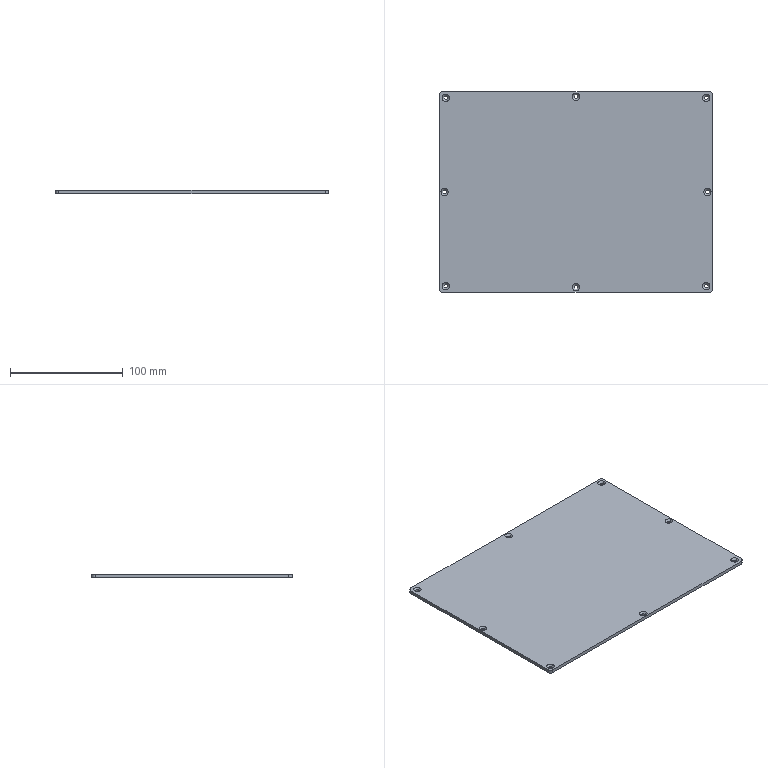Part | SolidWorks | features Extrusion 1, Fillet 1, HoleWzd 1 | 1 solid | 42 faces | box 242 x 178 x 3 mm | volume 128843 mm3 | cylinder 20 | cone 16 | plane 6 | commonest cylinder face diameters 3.4 x16 6 x4
STEP:
#1=CARTESIAN_POINT('',(-1.7,84.5,1.4));
#2=VERTEX_POINT('',#1);
#3=CARTESIAN_POINT('',(1.7,84.5,1.4));
#4=VERTEX_POINT('',#3);
#5=CARTESIAN_POINT('',(0.,84.5,1.4));
#6=DIRECTION('',(0.,0.,1.));
#7=DIRECTION('',(1.,0.,0.));
#8=AXIS2_PLACEMENT_3D('',#5,#6,#7);
#9=CIRCLE('',#8,1.7);
#10=EDGE_CURVE('',#2,#4,#9,.T.);
#11=ORIENTED_EDGE('',*,*,#10,.F.);
#12=CARTESIAN_POINT('',(-3.3,84.5,3.));
#13=VERTEX_POINT('',#12);
#14=CARTESIAN_POINT('',(-3.3,84.5,3.));
#15=DIRECTION('',(-0.7071,0.,0.7071));
#16=VECTOR('',#15,1000.);
#17=LINE('',#14,#16);
#18=EDGE_CURVE('',#2,#13,#17,.T.);
#19=ORIENTED_EDGE('',*,*,#18,.T.);
#20=CARTESIAN_POINT('',(3.3,84.5,3.));
#21=VERTEX_POINT('',#20);
#22=CARTESIAN_POINT('',(0.,84.5,3.));
#23=DIRECTION('',(0.,0.,1.));
#24=DIRECTION('',(1.,0.,0.));
#25=AXIS2_PLACEMENT_3D('',#22,#23,#24);
#26=CIRCLE('',#25,3.3);
#27=EDGE_CURVE('',#13,#21,#26,.T.);
#28=ORIENTED_EDGE('',*,*,#27,.T.);
#29=CARTESIAN_POINT('',(3.3,84.5,3.));
#30=DIRECTION('',(0.7071,0.,0.7071));
#31=VECTOR('',#30,1000.);
#32=LINE('',#29,#31);
#33=EDGE_CURVE('',#4,#21,#32,.T.);
#34=ORIENTED_EDGE('',*,*,#33,.F.);
#35=EDGE_LOOP('',(#11,#19,#28,#34));
#36=FACE_OUTER_BOUND('',#35,.T.);
#37=CARTESIAN_POINT('',(0.,84.5,3.));
#38=DIRECTION('',(0.,0.,1.));
#39=DIRECTION('',(1.,0.,0.));
#40=AXIS2_PLACEMENT_3D('',#37,#38,#39);
#41=CONICAL_SURFACE('',#40,3.3,0.7854);
#42=ADVANCED_FACE('',(#36),#41,.F.);
#43=CARTESIAN_POINT('',(-1.7,84.5,0.));
#44=VERTEX_POINT('',#43);
#45=CARTESIAN_POINT('',(1.7,84.5,0.));
#46=VERTEX_POINT('',#45);
#47=CARTESIAN_POINT('',(0.,84.5,0.));
#48=DIRECTION('',(0.,0.,1.));
#49=DIRECTION('',(1.,0.,0.));
#50=AXIS2_PLACEMENT_3D('',#47,#48,#49);
#51=CIRCLE('',#50,1.7);
#52=EDGE_CURVE('',#44,#46,#51,.T.);
#53=ORIENTED_EDGE('',*,*,#52,.F.);
#54=CARTESIAN_POINT('',(-1.7,84.5,3.));
#55=DIRECTION('',(0.,0.,1.));
#56=VECTOR('',#55,1000.);
#57=LINE('',#54,#56);
#58=EDGE_CURVE('',#44,#2,#57,.T.);
#59=ORIENTED_EDGE('',*,*,#58,.T.);
#60=ORIENTED_EDGE('',*,*,#10,.T.);
#61=CARTESIAN_POINT('',(1.7,84.5,3.));
#62=DIRECTION('',(0.,0.,1.));
#63=VECTOR('',#62,1000.);
#64=LINE('',#61,#63);
#65=EDGE_CURVE('',#46,#4,#64,.T.);
#66=ORIENTED_EDGE('',*,*,#65,.F.);
#67=EDGE_LOOP('',(#53,#59,#60,#66));
#68=FACE_OUTER_BOUND('',#67,.T.);
#69=CARTESIAN_POINT('',(0.,84.5,3.));
#70=DIRECTION('',(0.,0.,1.));
#71=DIRECTION('',(1.,0.,0.));
#72=AXIS2_PLACEMENT_3D('',#69,#70,#71);
#73=CYLINDRICAL_SURFACE('',#72,1.7);
#74=ADVANCED_FACE('',(#68),#73,.F.);
#75=CARTESIAN_POINT('',(-118.2,0.,1.4));
#76=VERTEX_POINT('',#75);
#77=CARTESIAN_POINT('',(-114.8,0.,1.4));
#78=VERTEX_POINT('',#77);
#79=CARTESIAN_POINT('',(-116.5,0.,1.4));
#80=DIRECTION('',(0.,0.,1.));
#81=DIRECTION('',(1.,0.,0.));
#82=AXIS2_PLACEMENT_3D('',#79,#80,#81);
#83=CIRCLE('',#82,1.7);
#84=EDGE_CURVE('',#76,#78,#83,.T.);
#85=ORIENTED_EDGE('',*,*,#84,.F.);
#86=CARTESIAN_POINT('',(-119.8,0.,3.));
#87=VERTEX_POINT('',#86);
#88=CARTESIAN_POINT('',(-119.8,0.,3.));
#89=DIRECTION('',(-0.7071,0.,0.7071));
#90=VECTOR('',#89,1000.);
#91=LINE('',#88,#90);
#92=EDGE_CURVE('',#76,#87,#91,.T.);
#93=ORIENTED_EDGE('',*,*,#92,.T.);
#94=CARTESIAN_POINT('',(-113.2,0.,3.));
#95=VERTEX_POINT('',#94);
#96=CARTESIAN_POINT('',(-116.5,0.,3.));
#97=DIRECTION('',(0.,0.,1.));
#98=DIRECTION('',(1.,0.,0.));
#99=AXIS2_PLACEMENT_3D('',#96,#97,#98);
#100=CIRCLE('',#99,3.3);
#101=EDGE_CURVE('',#87,#95,#100,.T.);
#102=ORIENTED_EDGE('',*,*,#101,.T.);
#103=CARTESIAN_POINT('',(-113.2,0.,3.));
#104=DIRECTION('',(0.7071,0.,0.7071));
#105=VECTOR('',#104,1000.);
#106=LINE('',#103,#105);
#107=EDGE_CURVE('',#78,#95,#106,.T.);
#108=ORIENTED_EDGE('',*,*,#107,.F.);
#109=EDGE_LOOP('',(#85,#93,#102,#108));
#110=FACE_OUTER_BOUND('',#109,.T.);
#111=CARTESIAN_POINT('',(-116.5,0.,3.));
#112=DIRECTION('',(0.,0.,1.));
#113=DIRECTION('',(1.,0.,0.));
#114=AXIS2_PLACEMENT_3D('',#111,#112,#113);
#115=CONICAL_SURFACE('',#114,3.3,0.7854);
#116=ADVANCED_FACE('',(#110),#115,.F.);
#117=CARTESIAN_POINT('',(-118.2,0.,0.));
#118=VERTEX_POINT('',#117);
#119=CARTESIAN_POINT('',(-114.8,0.,0.));
#120=VERTEX_POINT('',#119);
#121=CARTESIAN_POINT('',(-116.5,0.,0.));
#122=DIRECTION('',(0.,0.,1.));
#123=DIRECTION('',(1.,0.,0.));
#124=AXIS2_PLACEMENT_3D('',#121,#122,#123);
#125=CIRCLE('',#124,1.7);
#126=EDGE_CURVE('',#118,#120,#125,.T.);
#127=ORIENTED_EDGE('',*,*,#126,.F.);
#128=CARTESIAN_POINT('',(-118.2,0.,3.));
#129=DIRECTION('',(0.,0.,1.));
#130=VECTOR('',#129,1000.);
#131=LINE('',#128,#130);
#132=EDGE_CURVE('',#118,#76,#131,.T.);
#133=ORIENTED_EDGE('',*,*,#132,.T.);
#134=ORIENTED_EDGE('',*,*,#84,.T.);
#135=CARTESIAN_POINT('',(-114.8,0.,3.));
#136=DIRECTION('',(0.,0.,1.));
#137=VECTOR('',#136,1000.);
#138=LINE('',#135,#137);
#139=EDGE_CURVE('',#120,#78,#138,.T.);
#140=ORIENTED_EDGE('',*,*,#139,.F.);
#141=EDGE_LOOP('',(#127,#133,#134,#140));
#142=FACE_OUTER_BOUND('',#141,.T.);
#143=CARTESIAN_POINT('',(-116.5,0.,3.));
#144=DIRECTION('',(0.,0.,1.));
#145=DIRECTION('',(1.,0.,0.));
#146=AXIS2_PLACEMENT_3D('',#143,#144,#145);
#147=CYLINDRICAL_SURFACE('',#146,1.7);
#148=ADVANCED_FACE('',(#142),#147,.F.);
#149=CARTESIAN_POINT('',(-1.7,-84.5,1.4));
#150=VERTEX_POINT('',#149);
#151=CARTESIAN_POINT('',(1.7,-84.5,1.4));
#152=VERTEX_POINT('',#151);
#153=CARTESIAN_POINT('',(0.,-84.5,1.4));
#154=DIRECTION('',(0.,0.,1.));
#155=DIRECTION('',(1.,0.,0.));
#156=AXIS2_PLACEMENT_3D('',#153,#154,#155);
#157=CIRCLE('',#156,1.7);
#158=EDGE_CURVE('',#150,#152,#157,.T.);
#159=ORIENTED_EDGE('',*,*,#158,.F.);
#160=CARTESIAN_POINT('',(-3.3,-84.5,3.));
#161=VERTEX_POINT('',#160);
#162=CARTESIAN_POINT('',(-3.3,-84.5,3.));
#163=DIRECTION('',(-0.7071,0.,0.7071));
#164=VECTOR('',#163,1000.);
#165=LINE('',#162,#164);
#166=EDGE_CURVE('',#150,#161,#165,.T.);
#167=ORIENTED_EDGE('',*,*,#166,.T.);
#168=CARTESIAN_POINT('',(3.3,-84.5,3.));
#169=VERTEX_POINT('',#168);
#170=CARTESIAN_POINT('',(0.,-84.5,3.));
#171=DIRECTION('',(0.,0.,1.));
#172=DIRECTION('',(1.,0.,0.));
#173=AXIS2_PLACEMENT_3D('',#170,#171,#172);
#174=CIRCLE('',#173,3.3);
#175=EDGE_CURVE('',#161,#169,#174,.T.);
#176=ORIENTED_EDGE('',*,*,#175,.T.);
#177=CARTESIAN_POINT('',(3.3,-84.5,3.));
#178=DIRECTION('',(0.7071,0.,0.7071));
#179=VECTOR('',#178,1000.);
#180=LINE('',#177,#179);
#181=EDGE_CURVE('',#152,#169,#180,.T.);
#182=ORIENTED_EDGE('',*,*,#181,.F.);
#183=EDGE_LOOP('',(#159,#167,#176,#182));
#184=FACE_OUTER_BOUND('',#183,.T.);
#185=CARTESIAN_POINT('',(0.,-84.5,3.));
#186=DIRECTION('',(0.,0.,1.));
#187=DIRECTION('',(1.,0.,0.));
#188=AXIS2_PLACEMENT_3D('',#185,#186,#187);
#189=CONICAL_SURFACE('',#188,3.3,0.7854);
#190=ADVANCED_FACE('',(#184),#189,.F.);
#191=CARTESIAN_POINT('',(-1.7,-84.5,0.));
#192=VERTEX_POINT('',#191);
#193=CARTESIAN_POINT('',(1.7,-84.5,0.));
#194=VERTEX_POINT('',#193);
#195=CARTESIAN_POINT('',(0.,-84.5,0.));
#196=DIRECTION('',(0.,0.,1.));
#197=DIRECTION('',(1.,0.,0.));
#198=AXIS2_PLACEMENT_3D('',#195,#196,#197);
#199=CIRCLE('',#198,1.7);
#200=EDGE_CURVE('',#192,#194,#199,.T.);
#201=ORIENTED_EDGE('',*,*,#200,.F.);
#202=CARTESIAN_POINT('',(-1.7,-84.5,3.));
#203=DIRECTION('',(0.,0.,1.));
#204=VECTOR('',#203,1000.);
#205=LINE('',#202,#204);
#206=EDGE_CURVE('',#192,#150,#205,.T.);
#207=ORIENTED_EDGE('',*,*,#206,.T.);
#208=ORIENTED_EDGE('',*,*,#158,.T.);
#209=CARTESIAN_POINT('',(1.7,-84.5,3.));
#210=DIRECTION('',(0.,0.,1.));
#211=VECTOR('',#210,1000.);
#212=LINE('',#209,#211);
#213=EDGE_CURVE('',#194,#152,#212,.T.);
#214=ORIENTED_EDGE('',*,*,#213,.F.);
#215=EDGE_LOOP('',(#201,#207,#208,#214));
#216=FACE_OUTER_BOUND('',#215,.T.);
#217=CARTESIAN_POINT('',(0.,-84.5,3.));
#218=DIRECTION('',(0.,0.,1.));
#219=DIRECTION('',(1.,0.,0.));
#220=AXIS2_PLACEMENT_3D('',#217,#218,#219);
#221=CYLINDRICAL_SURFACE('',#220,1.7);
#222=ADVANCED_FACE('',(#216),#221,.F.);
#223=CARTESIAN_POINT('',(114.8,0.,1.4));
#224=VERTEX_POINT('',#223);
#225=CARTESIAN_POINT('',(118.2,0.,1.4));
#226=VERTEX_POINT('',#225);
#227=CARTESIAN_POINT('',(116.5,0.,1.4));
#228=DIRECTION('',(0.,0.,1.));
#229=DIRECTION('',(1.,0.,0.));
#230=AXIS2_PLACEMENT_3D('',#227,#228,#229);
#231=CIRCLE('',#230,1.7);
#232=EDGE_CURVE('',#224,#226,#231,.T.);
#233=ORIENTED_EDGE('',*,*,#232,.F.);
#234=CARTESIAN_POINT('',(113.2,0.,3.));
#235=VERTEX_POINT('',#234);
#236=CARTESIAN_POINT('',(113.2,0.,3.));
#237=DIRECTION('',(-0.7071,0.,0.7071));
#238=VECTOR('',#237,1000.);
#239=LINE('',#236,#238);
#240=EDGE_CURVE('',#224,#235,#239,.T.);
#241=ORIENTED_EDGE('',*,*,#240,.T.);
#242=CARTESIAN_POINT('',(119.8,0.,3.));
#243=VERTEX_POINT('',#242);
#244=CARTESIAN_POINT('',(116.5,0.,3.));
#245=DIRECTION('',(0.,0.,1.));
#246=DIRECTION('',(1.,0.,0.));
#247=AXIS2_PLACEMENT_3D('',#244,#245,#246);
#248=CIRCLE('',#247,3.3);
#249=EDGE_CURVE('',#235,#243,#248,.T.);
#250=ORIENTED_EDGE('',*,*,#249,.T.);
#251=CARTESIAN_POINT('',(119.8,0.,3.));
#252=DIRECTION('',(0.7071,0.,0.7071));
#253=VECTOR('',#252,1000.);
#254=LINE('',#251,#253);
#255=EDGE_CURVE('',#226,#243,#254,.T.);
#256=ORIENTED_EDGE('',*,*,#255,.F.);
#257=EDGE_LOOP('',(#233,#241,#250,#256));
#258=FACE_OUTER_BOUND('',#257,.T.);
#259=CARTESIAN_POINT('',(116.5,0.,3.));
#260=DIRECTION('',(0.,0.,1.));
#261=DIRECTION('',(1.,0.,0.));
#262=AXIS2_PLACEMENT_3D('',#259,#260,#261);
#263=CONICAL_SURFACE('',#262,3.3,0.7854);
#264=ADVANCED_FACE('',(#258),#263,.F.);
#265=CARTESIAN_POINT('',(114.8,0.,0.));
#266=VERTEX_POINT('',#265);
#267=CARTESIAN_POINT('',(118.2,0.,0.));
#268=VERTEX_POINT('',#267);
#269=CARTESIAN_POINT('',(116.5,0.,0.));
#270=DIRECTION('',(0.,0.,1.));
#271=DIRECTION('',(1.,0.,0.));
#272=AXIS2_PLACEMENT_3D('',#269,#270,#271);
#273=CIRCLE('',#272,1.7);
#274=EDGE_CURVE('',#266,#268,#273,.T.);
#275=ORIENTED_EDGE('',*,*,#274,.F.);
#276=CARTESIAN_POINT('',(114.8,0.,3.));
#277=DIRECTION('',(0.,0.,1.));
#278=VECTOR('',#277,1000.);
#279=LINE('',#276,#278);
#280=EDGE_CURVE('',#266,#224,#279,.T.);
#281=ORIENTED_EDGE('',*,*,#280,.T.);
#282=ORIENTED_EDGE('',*,*,#232,.T.);
#283=CARTESIAN_POINT('',(118.2,0.,3.));
#284=DIRECTION('',(0.,0.,1.));
#285=VECTOR('',#284,1000.);
#286=LINE('',#283,#285);
#287=EDGE_CURVE('',#268,#226,#286,.T.);
#288=ORIENTED_EDGE('',*,*,#287,.F.);
#289=EDGE_LOOP('',(#275,#281,#282,#288));
#290=FACE_OUTER_BOUND('',#289,.T.);
#291=CARTESIAN_POINT('',(116.5,0.,3.));
#292=DIRECTION('',(0.,0.,1.));
#293=DIRECTION('',(1.,0.,0.));
#294=AXIS2_PLACEMENT_3D('',#291,#292,#293);
#295=CYLINDRICAL_SURFACE('',#294,1.7);
#296=ADVANCED_FACE('',(#290),#295,.F.);
#297=CARTESIAN_POINT('',(-117.2,83.5,1.4));
#298=VERTEX_POINT('',#297);
#299=CARTESIAN_POINT('',(-113.8,83.5,1.4));
#300=VERTEX_POINT('',#299);
#301=CARTESIAN_POINT('',(-115.5,83.5,1.4));
#302=DIRECTION('',(0.,0.,1.));
#303=DIRECTION('',(1.,0.,0.));
#304=AXIS2_PLACEMENT_3D('',#301,#302,#303);
#305=CIRCLE('',#304,1.7);
#306=EDGE_CURVE('',#298,#300,#305,.T.);
#307=ORIENTED_EDGE('',*,*,#306,.F.);
#308=CARTESIAN_POINT('',(-118.8,83.5,3.));
#309=VERTEX_POINT('',#308);
#310=CARTESIAN_POINT('',(-118.8,83.5,3.));
#311=DIRECTION('',(-0.7071,0.,0.7071));
#312=VECTOR('',#311,1000.);
#313=LINE('',#310,#312);
#314=EDGE_CURVE('',#298,#309,#313,.T.);
#315=ORIENTED_EDGE('',*,*,#314,.T.);
#316=CARTESIAN_POINT('',(-112.2,83.5,3.));
#317=VERTEX_POINT('',#316);
#318=CARTESIAN_POINT('',(-115.5,83.5,3.));
#319=DIRECTION('',(0.,0.,1.));
#320=DIRECTION('',(1.,0.,0.));
#321=AXIS2_PLACEMENT_3D('',#318,#319,#320);
#322=CIRCLE('',#321,3.3);
#323=EDGE_CURVE('',#309,#317,#322,.T.);
#324=ORIENTED_EDGE('',*,*,#323,.T.);
#325=CARTESIAN_POINT('',(-112.2,83.5,3.));
#326=DIRECTION('',(0.7071,0.,0.7071));
#327=VECTOR('',#326,1000.);
#328=LINE('',#325,#327);
#329=EDGE_CURVE('',#300,#317,#328,.T.);
#330=ORIENTED_EDGE('',*,*,#329,.F.);
#331=EDGE_LOOP('',(#307,#315,#324,#330));
#332=FACE_OUTER_BOUND('',#331,.T.);
#333=CARTESIAN_POINT('',(-115.5,83.5,3.));
#334=DIRECTION('',(0.,0.,1.));
#335=DIRECTION('',(1.,0.,0.));
#336=AXIS2_PLACEMENT_3D('',#333,#334,#335);
#337=CONICAL_SURFACE('',#336,3.3,0.7854);
#338=ADVANCED_FACE('',(#332),#337,.F.);
#339=CARTESIAN_POINT('',(-117.2,83.5,0.));
#340=VERTEX_POINT('',#339);
#341=CARTESIAN_POINT('',(-113.8,83.5,0.));
#342=VERTEX_POINT('',#341);
#343=CARTESIAN_POINT('',(-115.5,83.5,0.));
#344=DIRECTION('',(0.,0.,1.));
#345=DIRECTION('',(1.,0.,0.));
#346=AXIS2_PLACEMENT_3D('',#343,#344,#345);
#347=CIRCLE('',#346,1.7);
#348=EDGE_CURVE('',#340,#342,#347,.T.);
#349=ORIENTED_EDGE('',*,*,#348,.F.);
#350=CARTESIAN_POINT('',(-117.2,83.5,3.));
#351=DIRECTION('',(0.,0.,1.));
#352=VECTOR('',#351,1000.);
#353=LINE('',#350,#352);
#354=EDGE_CURVE('',#340,#298,#353,.T.);
#355=ORIENTED_EDGE('',*,*,#354,.T.);
#356=ORIENTED_EDGE('',*,*,#306,.T.);
#357=CARTESIAN_POINT('',(-113.8,83.5,3.));
#358=DIRECTION('',(0.,0.,1.));
#359=VECTOR('',#358,1000.);
#360=LINE('',#357,#359);
#361=EDGE_CURVE('',#342,#300,#360,.T.);
#362=ORIENTED_EDGE('',*,*,#361,.F.);
#363=EDGE_LOOP('',(#349,#355,#356,#362));
#364=FACE_OUTER_BOUND('',#363,.T.);
#365=CARTESIAN_POINT('',(-115.5,83.5,3.));
#366=DIRECTION('',(0.,0.,1.));
#367=DIRECTION('',(1.,0.,0.));
#368=AXIS2_PLACEMENT_3D('',#365,#366,#367);
#369=CYLINDRICAL_SURFACE('',#368,1.7);
#370=ADVANCED_FACE('',(#364),#369,.F.);
#371=CARTESIAN_POINT('',(-117.2,-83.5,1.4));
#372=VERTEX_POINT('',#371);
#373=CARTESIAN_POINT('',(-113.8,-83.5,1.4));
#374=VERTEX_POINT('',#373);
#375=CARTESIAN_POINT('',(-115.5,-83.5,1.4));
#376=DIRECTION('',(0.,0.,1.));
#377=DIRECTION('',(1.,0.,0.));
#378=AXIS2_PLACEMENT_3D('',#375,#376,#377);
#379=CIRCLE('',#378,1.7);
#380=EDGE_CURVE('',#372,#374,#379,.T.);
#381=ORIENTED_EDGE('',*,*,#380,.F.);
#382=CARTESIAN_POINT('',(-118.8,-83.5,3.));
#383=VERTEX_POINT('',#382);
#384=CARTESIAN_POINT('',(-118.8,-83.5,3.));
#385=DIRECTION('',(-0.7071,0.,0.7071));
#386=VECTOR('',#385,1000.);
#387=LINE('',#384,#386);
#388=EDGE_CURVE('',#372,#383,#387,.T.);
#389=ORIENTED_EDGE('',*,*,#388,.T.);
#390=CARTESIAN_POINT('',(-112.2,-83.5,3.));
#391=VERTEX_POINT('',#390);
#392=CARTESIAN_POINT('',(-115.5,-83.5,3.));
#393=DIRECTION('',(0.,0.,1.));
#394=DIRECTION('',(1.,0.,0.));
#395=AXIS2_PLACEMENT_3D('',#392,#393,#394);
#396=CIRCLE('',#395,3.3);
#397=EDGE_CURVE('',#383,#391,#396,.T.);
#398=ORIENTED_EDGE('',*,*,#397,.T.);
#399=CARTESIAN_POINT('',(-112.2,-83.5,3.));
#400=DIRECTION('',(0.7071,0.,0.7071));
#401=VECTOR('',#400,1000.);
#402=LINE('',#399,#401);
#403=EDGE_CURVE('',#374,#391,#402,.T.);
#404=ORIENTED_EDGE('',*,*,#403,.F.);
#405=EDGE_LOOP('',(#381,#389,#398,#404));
#406=FACE_OUTER_BOUND('',#405,.T.);
#407=CARTESIAN_POINT('',(-115.5,-83.5,3.));
#408=DIRECTION('',(0.,0.,1.));
#409=DIRECTION('',(1.,0.,0.));
#410=AXIS2_PLACEMENT_3D('',#407,#408,#409);
#411=CONICAL_SURFACE('',#410,3.3,0.7854);
#412=ADVANCED_FACE('',(#406),#411,.F.);
#413=CARTESIAN_POINT('',(-117.2,-83.5,0.));
#414=VERTEX_POINT('',#413);
#415=CARTESIAN_POINT('',(-113.8,-83.5,0.));
#416=VERTEX_POINT('',#415);
#417=CARTESIAN_POINT('',(-115.5,-83.5,0.));
#418=DIRECTION('',(0.,0.,1.));
#419=DIRECTION('',(1.,0.,0.));
#420=AXIS2_PLACEMENT_3D('',#417,#418,#419);
#421=CIRCLE('',#420,1.7);
#422=EDGE_CURVE('',#414,#416,#421,.T.);
#423=ORIENTED_EDGE('',*,*,#422,.F.);
#424=CARTESIAN_POINT('',(-117.2,-83.5,3.));
#425=DIRECTION('',(0.,0.,1.));
#426=VECTOR('',#425,1000.);
#427=LINE('',#424,#426);
#428=EDGE_CURVE('',#414,#372,#427,.T.);
#429=ORIENTED_EDGE('',*,*,#428,.T.);
#430=ORIENTED_EDGE('',*,*,#380,.T.);
#431=CARTESIAN_POINT('',(-113.8,-83.5,3.));
#432=DIRECTION('',(0.,0.,1.));
#433=VECTOR('',#432,1000.);
#434=LINE('',#431,#433);
#435=EDGE_CURVE('',#416,#374,#434,.T.);
#436=ORIENTED_EDGE('',*,*,#435,.F.);
#437=EDGE_LOOP('',(#423,#429,#430,#436));
#438=FACE_OUTER_BOUND('',#437,.T.);
#439=CARTESIAN_POINT('',(-115.5,-83.5,3.));
#440=DIRECTION('',(0.,0.,1.));
#441=DIRECTION('',(1.,0.,0.));
#442=AXIS2_PLACEMENT_3D('',#439,#440,#441);
#443=CYLINDRICAL_SURFACE('',#442,1.7);
#444=ADVANCED_FACE('',(#438),#443,.F.);
#445=CARTESIAN_POINT('',(113.8,-83.5,1.4));
#446=VERTEX_POINT('',#445);
#447=CARTESIAN_POINT('',(117.2,-83.5,1.4));
#448=VERTEX_POINT('',#447);
#449=CARTESIAN_POINT('',(115.5,-83.5,1.4));
#450=DIRECTION('',(0.,0.,1.));
#451=DIRECTION('',(1.,0.,0.));
#452=AXIS2_PLACEMENT_3D('',#449,#450,#451);
#453=CIRCLE('',#452,1.7);
#454=EDGE_CURVE('',#446,#448,#453,.T.);
#455=ORIENTED_EDGE('',*,*,#454,.F.);
#456=CARTESIAN_POINT('',(112.2,-83.5,3.));
#457=VERTEX_POINT('',#456);
#458=CARTESIAN_POINT('',(112.2,-83.5,3.));
#459=DIRECTION('',(-0.7071,0.,0.7071));
#460=VECTOR('',#459,1000.);
#461=LINE('',#458,#460);
#462=EDGE_CURVE('',#446,#457,#461,.T.);
#463=ORIENTED_EDGE('',*,*,#462,.T.);
#464=CARTESIAN_POINT('',(118.8,-83.5,3.));
#465=VERTEX_POINT('',#464);
#466=CARTESIAN_POINT('',(115.5,-83.5,3.));
#467=DIRECTION('',(0.,0.,1.));
#468=DIRECTION('',(1.,0.,0.));
#469=AXIS2_PLACEMENT_3D('',#466,#467,#468);
#470=CIRCLE('',#469,3.3);
#471=EDGE_CURVE('',#457,#465,#470,.T.);
#472=ORIENTED_EDGE('',*,*,#471,.T.);
#473=CARTESIAN_POINT('',(118.8,-83.5,3.));
#474=DIRECTION('',(0.7071,0.,0.7071));
#475=VECTOR('',#474,1000.);
#476=LINE('',#473,#475);
#477=EDGE_CURVE('',#448,#465,#476,.T.);
#478=ORIENTED_EDGE('',*,*,#477,.F.);
#479=EDGE_LOOP('',(#455,#463,#472,#478));
#480=FACE_OUTER_BOUND('',#479,.T.);
#481=CARTESIAN_POINT('',(115.5,-83.5,3.));
#482=DIRECTION('',(0.,0.,1.));
#483=DIRECTION('',(1.,0.,0.));
#484=AXIS2_PLACEMENT_3D('',#481,#482,#483);
#485=CONICAL_SURFACE('',#484,3.3,0.7854);
#486=ADVANCED_FACE('',(#480),#485,.F.);
#487=CARTESIAN_POINT('',(113.8,-83.5,0.));
#488=VERTEX_POINT('',#487);
#489=CARTESIAN_POINT('',(117.2,-83.5,0.));
#490=VERTEX_POINT('',#489);
#491=CARTESIAN_POINT('',(115.5,-83.5,0.));
#492=DIRECTION('',(0.,0.,1.));
#493=DIRECTION('',(1.,0.,0.));
#494=AXIS2_PLACEMENT_3D('',#491,#492,#493);
#495=CIRCLE('',#494,1.7);
#496=EDGE_CURVE('',#488,#490,#495,.T.);
#497=ORIENTED_EDGE('',*,*,#496,.F.);
#498=CARTESIAN_POINT('',(113.8,-83.5,3.));
#499=DIRECTION('',(0.,0.,1.));
#500=VECTOR('',#499,1000.);
#501=LINE('',#498,#500);
#502=EDGE_CURVE('',#488,#446,#501,.T.);
#503=ORIENTED_EDGE('',*,*,#502,.T.);
#504=ORIENTED_EDGE('',*,*,#454,.T.);
#505=CARTESIAN_POINT('',(117.2,-83.5,3.));
#506=DIRECTION('',(0.,0.,1.));
#507=VECTOR('',#506,1000.);
#508=LINE('',#505,#507);
#509=EDGE_CURVE('',#490,#448,#508,.T.);
#510=ORIENTED_EDGE('',*,*,#509,.F.);
#511=EDGE_LOOP('',(#497,#503,#504,#510));
#512=FACE_OUTER_BOUND('',#511,.T.);
#513=CARTESIAN_POINT('',(115.5,-83.5,3.));
#514=DIRECTION('',(0.,0.,1.));
#515=DIRECTION('',(1.,0.,0.));
#516=AXIS2_PLACEMENT_3D('',#513,#514,#515);
#517=CYLINDRICAL_SURFACE('',#516,1.7);
#518=ADVANCED_FACE('',(#512),#517,.F.);
#519=CARTESIAN_POINT('',(113.8,83.5,1.4));
#520=VERTEX_POINT('',#519);
#521=CARTESIAN_POINT('',(117.2,83.5,1.4));
#522=VERTEX_POINT('',#521);
#523=CARTESIAN_POINT('',(115.5,83.5,1.4));
#524=DIRECTION('',(0.,0.,1.));
#525=DIRECTION('',(1.,0.,0.));
#526=AXIS2_PLACEMENT_3D('',#523,#524,#525);
#527=CIRCLE('',#526,1.7);
#528=EDGE_CURVE('',#520,#522,#527,.T.);
#529=ORIENTED_EDGE('',*,*,#528,.F.);
#530=CARTESIAN_POINT('',(112.2,83.5,3.));
#531=VERTEX_POINT('',#530);
#532=CARTESIAN_POINT('',(112.2,83.5,3.));
#533=DIRECTION('',(-0.7071,0.,0.7071));
#534=VECTOR('',#533,1000.);
#535=LINE('',#532,#534);
#536=EDGE_CURVE('',#520,#531,#535,.T.);
#537=ORIENTED_EDGE('',*,*,#536,.T.);
#538=CARTESIAN_POINT('',(118.8,83.5,3.));
#539=VERTEX_POINT('',#538);
#540=CARTESIAN_POINT('',(115.5,83.5,3.));
#541=DIRECTION('',(0.,0.,1.));
#542=DIRECTION('',(1.,0.,0.));
#543=AXIS2_PLACEMENT_3D('',#540,#541,#542);
#544=CIRCLE('',#543,3.3);
#545=EDGE_CURVE('',#531,#539,#544,.T.);
#546=ORIENTED_EDGE('',*,*,#545,.T.);
#547=CARTESIAN_POINT('',(118.8,83.5,3.));
#548=DIRECTION('',(0.7071,0.,0.7071));
#549=VECTOR('',#548,1000.);
#550=LINE('',#547,#549);
#551=EDGE_CURVE('',#522,#539,#550,.T.);
#552=ORIENTED_EDGE('',*,*,#551,.F.);
#553=EDGE_LOOP('',(#529,#537,#546,#552));
#554=FACE_OUTER_BOUND('',#553,.T.);
#555=CARTESIAN_POINT('',(115.5,83.5,3.));
#556=DIRECTION('',(0.,0.,1.));
#557=DIRECTION('',(1.,0.,0.));
#558=AXIS2_PLACEMENT_3D('',#555,#556,#557);
#559=CONICAL_SURFACE('',#558,3.3,0.7854);
#560=ADVANCED_FACE('',(#554),#559,.F.);
#561=CARTESIAN_POINT('',(113.8,83.5,0.));
#562=VERTEX_POINT('',#561);
#563=CARTESIAN_POINT('',(117.2,83.5,0.));
#564=VERTEX_POINT('',#563);
#565=CARTESIAN_POINT('',(115.5,83.5,0.));
#566=DIRECTION('',(0.,0.,1.));
#567=DIRECTION('',(1.,0.,0.));
#568=AXIS2_PLACEMENT_3D('',#565,#566,#567);
#569=CIRCLE('',#568,1.7);
#570=EDGE_CURVE('',#562,#564,#569,.T.);
#571=ORIENTED_EDGE('',*,*,#570,.F.);
#572=CARTESIAN_POINT('',(113.8,83.5,3.));
#573=DIRECTION('',(0.,0.,1.));
#574=VECTOR('',#573,1000.);
#575=LINE('',#572,#574);
#576=EDGE_CURVE('',#562,#520,#575,.T.);
#577=ORIENTED_EDGE('',*,*,#576,.T.);
#578=ORIENTED_EDGE('',*,*,#528,.T.);
#579=CARTESIAN_POINT('',(117.2,83.5,3.));
#580=DIRECTION('',(0.,0.,1.));
#581=VECTOR('',#580,1000.);
#582=LINE('',#579,#581);
#583=EDGE_CURVE('',#564,#522,#582,.T.);
#584=ORIENTED_EDGE('',*,*,#583,.F.);
#585=EDGE_LOOP('',(#571,#577,#578,#584));
#586=FACE_OUTER_BOUND('',#585,.T.);
#587=CARTESIAN_POINT('',(115.5,83.5,3.));
#588=DIRECTION('',(0.,0.,1.));
#589=DIRECTION('',(1.,0.,0.));
#590=AXIS2_PLACEMENT_3D('',#587,#588,#589);
#591=CYLINDRICAL_SURFACE('',#590,1.7);
#592=ADVANCED_FACE('',(#586),#591,.F.);
#593=CARTESIAN_POINT('',(121.,-86.,3.));
#594=VERTEX_POINT('',#593);
#595=CARTESIAN_POINT('',(121.,86.,3.));
#596=VERTEX_POINT('',#595);
#597=CARTESIAN_POINT('',(121.,89.,3.));
#598=DIRECTION('',(0.,1.,0.));
#599=VECTOR('',#598,1000.);
#600=LINE('',#597,#599);
#601=EDGE_CURVE('',#594,#596,#600,.T.);
#602=ORIENTED_EDGE('',*,*,#601,.F.);
#603=CARTESIAN_POINT('',(121.,-86.,0.));
#604=VERTEX_POINT('',#603);
#605=CARTESIAN_POINT('',(121.,-86.,3.));
#606=DIRECTION('',(0.,0.,-1.));
#607=VECTOR('',#606,1000.);
#608=LINE('',#605,#607);
#609=EDGE_CURVE('',#594,#604,#608,.T.);
#610=ORIENTED_EDGE('',*,*,#609,.T.);
#611=CARTESIAN_POINT('',(121.,86.,0.));
#612=VERTEX_POINT('',#611);
#613=CARTESIAN_POINT('',(121.,89.,0.));
#614=DIRECTION('',(0.,1.,0.));
#615=VECTOR('',#614,1000.);
#616=LINE('',#613,#615);
#617=EDGE_CURVE('',#604,#612,#616,.T.);
#618=ORIENTED_EDGE('',*,*,#617,.T.);
#619=CARTESIAN_POINT('',(121.,86.,3.));
#620=DIRECTION('',(0.,0.,1.));
#621=VECTOR('',#620,1000.);
#622=LINE('',#619,#621);
#623=EDGE_CURVE('',#612,#596,#622,.T.);
#624=ORIENTED_EDGE('',*,*,#623,.T.);
#625=EDGE_LOOP('',(#602,#610,#618,#624));
#626=FACE_OUTER_BOUND('',#625,.T.);
#627=CARTESIAN_POINT('',(121.,89.,3.));
#628=DIRECTION('',(-1.,0.,0.));
#629=DIRECTION('',(0.,-1.,0.));
#630=AXIS2_PLACEMENT_3D('',#627,#628,#629);
#631=PLANE('',#630);
#632=ADVANCED_FACE('',(#626),#631,.F.);
#633=CARTESIAN_POINT('',(118.,89.,3.));
#634=VERTEX_POINT('',#633);
#635=CARTESIAN_POINT('',(-118.,89.,3.));
#636=VERTEX_POINT('',#635);
#637=CARTESIAN_POINT('',(-121.,89.,3.));
#638=DIRECTION('',(-1.,0.,0.));
#639=VECTOR('',#638,1000.);
#640=LINE('',#637,#639);
#641=EDGE_CURVE('',#634,#636,#640,.T.);
#642=ORIENTED_EDGE('',*,*,#641,.F.);
#643=CARTESIAN_POINT('',(118.,89.,0.));
#644=VERTEX_POINT('',#643);
#645=CARTESIAN_POINT('',(118.,89.,3.));
#646=DIRECTION('',(0.,0.,-1.));
#647=VECTOR('',#646,1000.);
#648=LINE('',#645,#647);
#649=EDGE_CURVE('',#634,#644,#648,.T.);
#650=ORIENTED_EDGE('',*,*,#649,.T.);
#651=CARTESIAN_POINT('',(-118.,89.,0.));
#652=VERTEX_POINT('',#651);
#653=CARTESIAN_POINT('',(-121.,89.,0.));
#654=DIRECTION('',(-1.,0.,0.));
#655=VECTOR('',#654,1000.);
#656=LINE('',#653,#655);
#657=EDGE_CURVE('',#644,#652,#656,.T.);
#658=ORIENTED_EDGE('',*,*,#657,.T.);
#659=CARTESIAN_POINT('',(-118.,89.,3.));
#660=DIRECTION('',(0.,0.,1.));
#661=VECTOR('',#660,1000.);
#662=LINE('',#659,#661);
#663=EDGE_CURVE('',#652,#636,#662,.T.);
#664=ORIENTED_EDGE('',*,*,#663,.T.);
#665=EDGE_LOOP('',(#642,#650,#658,#664));
#666=FACE_OUTER_BOUND('',#665,.T.);
#667=CARTESIAN_POINT('',(-121.,89.,3.));
#668=DIRECTION('',(0.,-1.,0.));
#669=DIRECTION('',(0.,0.,-1.));
#670=AXIS2_PLACEMENT_3D('',#667,#668,#669);
#671=PLANE('',#670);
#672=ADVANCED_FACE('',(#666),#671,.F.);
#673=CARTESIAN_POINT('',(-121.,86.,0.));
#674=VERTEX_POINT('',#673);
#675=CARTESIAN_POINT('',(-121.,-86.,0.));
#676=VERTEX_POINT('',#675);
#677=CARTESIAN_POINT('',(-121.,89.,0.));
#678=DIRECTION('',(0.,-1.,0.));
#679=VECTOR('',#678,1000.);
#680=LINE('',#677,#679);
#681=EDGE_CURVE('',#674,#676,#680,.T.);
#682=ORIENTED_EDGE('',*,*,#681,.T.);
#683=CARTESIAN_POINT('',(-121.,-86.,3.));
#684=VERTEX_POINT('',#683);
#685=CARTESIAN_POINT('',(-121.,-86.,3.));
#686=DIRECTION('',(0.,0.,1.));
#687=VECTOR('',#686,1000.);
#688=LINE('',#685,#687);
#689=EDGE_CURVE('',#676,#684,#688,.T.);
#690=ORIENTED_EDGE('',*,*,#689,.T.);
#691=CARTESIAN_POINT('',(-121.,86.,3.));
#692=VERTEX_POINT('',#691);
#693=CARTESIAN_POINT('',(-121.,89.,3.));
#694=DIRECTION('',(0.,-1.,0.));
#695=VECTOR('',#694,1000.);
#696=LINE('',#693,#695);
#697=EDGE_CURVE('',#692,#684,#696,.T.);
#698=ORIENTED_EDGE('',*,*,#697,.F.);
#699=CARTESIAN_POINT('',(-121.,86.,3.));
#700=DIRECTION('',(0.,0.,-1.));
#701=VECTOR('',#700,1000.);
#702=LINE('',#699,#701);
#703=EDGE_CURVE('',#692,#674,#702,.T.);
#704=ORIENTED_EDGE('',*,*,#703,.T.);
#705=EDGE_LOOP('',(#682,#690,#698,#704));
#706=FACE_OUTER_BOUND('',#705,.T.);
#707=CARTESIAN_POINT('',(-121.,89.,3.));
#708=DIRECTION('',(1.,0.,0.));
#709=DIRECTION('',(0.,1.,0.));
#710=AXIS2_PLACEMENT_3D('',#707,#708,#709);
#711=PLANE('',#710);
#712=ADVANCED_FACE('',(#706),#711,.F.);
#713=CARTESIAN_POINT('',(-118.,-89.,3.));
#714=VERTEX_POINT('',#713);
#715=CARTESIAN_POINT('',(118.,-89.,3.));
#716=VERTEX_POINT('',#715);
#717=CARTESIAN_POINT('',(-121.,-89.,3.));
#718=DIRECTION('',(1.,0.,0.));
#719=VECTOR('',#718,1000.);
#720=LINE('',#717,#719);
#721=EDGE_CURVE('',#714,#716,#720,.T.);
#722=ORIENTED_EDGE('',*,*,#721,.F.);
#723=CARTESIAN_POINT('',(-118.,-89.,0.));
#724=VERTEX_POINT('',#723);
#725=CARTESIAN_POINT('',(-118.,-89.,3.));
#726=DIRECTION('',(0.,0.,-1.));
#727=VECTOR('',#726,1000.);
#728=LINE('',#725,#727);
#729=EDGE_CURVE('',#714,#724,#728,.T.);
#730=ORIENTED_EDGE('',*,*,#729,.T.);
#731=CARTESIAN_POINT('',(118.,-89.,0.));
#732=VERTEX_POINT('',#731);
#733=CARTESIAN_POINT('',(-121.,-89.,0.));
#734=DIRECTION('',(1.,0.,0.));
#735=VECTOR('',#734,1000.);
#736=LINE('',#733,#735);
#737=EDGE_CURVE('',#724,#732,#736,.T.);
#738=ORIENTED_EDGE('',*,*,#737,.T.);
#739=CARTESIAN_POINT('',(118.,-89.,3.));
#740=DIRECTION('',(0.,0.,1.));
#741=VECTOR('',#740,1000.);
#742=LINE('',#739,#741);
#743=EDGE_CURVE('',#732,#716,#742,.T.);
#744=ORIENTED_EDGE('',*,*,#743,.T.);
#745=EDGE_LOOP('',(#722,#730,#738,#744));
#746=FACE_OUTER_BOUND('',#745,.T.);
#747=CARTESIAN_POINT('',(-121.,-89.,3.));
#748=DIRECTION('',(0.,1.,0.));
#749=DIRECTION('',(0.,0.,1.));
#750=AXIS2_PLACEMENT_3D('',#747,#748,#749);
#751=PLANE('',#750);
#752=ADVANCED_FACE('',(#746),#751,.F.);
#753=CARTESIAN_POINT('',(0.,84.5,3.));
#754=DIRECTION('',(0.,0.,1.));
#755=DIRECTION('',(1.,0.,0.));
#756=AXIS2_PLACEMENT_3D('',#753,#754,#755);
#757=CIRCLE('',#756,3.3);
#758=EDGE_CURVE('',#21,#13,#757,.T.);
#759=ORIENTED_EDGE('',*,*,#758,.F.);
#760=ORIENTED_EDGE('',*,*,#27,.F.);
#761=EDGE_LOOP('',(#759,#760));
#762=FACE_BOUND('',#761,.T.);
#763=CARTESIAN_POINT('',(-116.5,0.,3.));
#764=DIRECTION('',(0.,0.,1.));
#765=DIRECTION('',(1.,0.,0.));
#766=AXIS2_PLACEMENT_3D('',#763,#764,#765);
#767=CIRCLE('',#766,3.3);
#768=EDGE_CURVE('',#95,#87,#767,.T.);
#769=ORIENTED_EDGE('',*,*,#768,.F.);
#770=ORIENTED_EDGE('',*,*,#101,.F.);
#771=EDGE_LOOP('',(#769,#770));
#772=FACE_BOUND('',#771,.T.);
#773=CARTESIAN_POINT('',(0.,-84.5,3.));
#774=DIRECTION('',(0.,0.,1.));
#775=DIRECTION('',(1.,0.,0.));
#776=AXIS2_PLACEMENT_3D('',#773,#774,#775);
#777=CIRCLE('',#776,3.3);
#778=EDGE_CURVE('',#169,#161,#777,.T.);
#779=ORIENTED_EDGE('',*,*,#778,.F.);
#780=ORIENTED_EDGE('',*,*,#175,.F.);
#781=EDGE_LOOP('',(#779,#780));
#782=FACE_BOUND('',#781,.T.);
#783=CARTESIAN_POINT('',(116.5,0.,3.));
#784=DIRECTION('',(0.,0.,1.));
#785=DIRECTION('',(1.,0.,0.));
#786=AXIS2_PLACEMENT_3D('',#783,#784,#785);
#787=CIRCLE('',#786,3.3);
#788=EDGE_CURVE('',#243,#235,#787,.T.);
#789=ORIENTED_EDGE('',*,*,#788,.F.);
#790=ORIENTED_EDGE('',*,*,#249,.F.);
#791=EDGE_LOOP('',(#789,#790));
#792=FACE_BOUND('',#791,.T.);
#793=CARTESIAN_POINT('',(-115.5,83.5,3.));
#794=DIRECTION('',(0.,0.,1.));
#795=DIRECTION('',(1.,0.,0.));
#796=AXIS2_PLACEMENT_3D('',#793,#794,#795);
#797=CIRCLE('',#796,3.3);
#798=EDGE_CURVE('',#317,#309,#797,.T.);
#799=ORIENTED_EDGE('',*,*,#798,.F.);
#800=ORIENTED_EDGE('',*,*,#323,.F.);
#801=EDGE_LOOP('',(#799,#800));
#802=FACE_BOUND('',#801,.T.);
#803=CARTESIAN_POINT('',(-115.5,-83.5,3.));
#804=DIRECTION('',(0.,0.,1.));
#805=DIRECTION('',(1.,0.,0.));
#806=AXIS2_PLACEMENT_3D('',#803,#804,#805);
#807=CIRCLE('',#806,3.3);
#808=EDGE_CURVE('',#391,#383,#807,.T.);
#809=ORIENTED_EDGE('',*,*,#808,.F.);
#810=ORIENTED_EDGE('',*,*,#397,.F.);
#811=EDGE_LOOP('',(#809,#810));
#812=FACE_BOUND('',#811,.T.);
#813=CARTESIAN_POINT('',(115.5,-83.5,3.));
#814=DIRECTION('',(0.,0.,1.));
#815=DIRECTION('',(1.,0.,0.));
#816=AXIS2_PLACEMENT_3D('',#813,#814,#815);
#817=CIRCLE('',#816,3.3);
#818=EDGE_CURVE('',#465,#457,#817,.T.);
#819=ORIENTED_EDGE('',*,*,#818,.F.);
#820=ORIENTED_EDGE('',*,*,#471,.F.);
#821=EDGE_LOOP('',(#819,#820));
#822=FACE_BOUND('',#821,.T.);
#823=CARTESIAN_POINT('',(115.5,83.5,3.));
#824=DIRECTION('',(0.,0.,1.));
#825=DIRECTION('',(1.,0.,0.));
#826=AXIS2_PLACEMENT_3D('',#823,#824,#825);
#827=CIRCLE('',#826,3.3);
#828=EDGE_CURVE('',#539,#531,#827,.T.);
#829=ORIENTED_EDGE('',*,*,#828,.F.);
#830=ORIENTED_EDGE('',*,*,#545,.F.);
#831=EDGE_LOOP('',(#829,#830));
#832=FACE_BOUND('',#831,.T.);
#833=ORIENTED_EDGE('',*,*,#697,.T.);
#834=CARTESIAN_POINT('',(-118.,-86.,3.));
#835=DIRECTION('',(0.,0.,1.));
#836=DIRECTION('',(1.,0.,0.));
#837=AXIS2_PLACEMENT_3D('',#834,#835,#836);
#838=CIRCLE('',#837,3.);
#839=EDGE_CURVE('',#684,#714,#838,.T.);
#840=ORIENTED_EDGE('',*,*,#839,.T.);
#841=ORIENTED_EDGE('',*,*,#721,.T.);
#842=CARTESIAN_POINT('',(118.,-86.,3.));
#843=DIRECTION('',(0.,0.,1.));
#844=DIRECTION('',(1.,0.,0.));
#845=AXIS2_PLACEMENT_3D('',#842,#843,#844);
#846=CIRCLE('',#845,3.);
#847=EDGE_CURVE('',#716,#594,#846,.T.);
#848=ORIENTED_EDGE('',*,*,#847,.T.);
#849=ORIENTED_EDGE('',*,*,#601,.T.);
#850=CARTESIAN_POINT('',(118.,86.,3.));
#851=DIRECTION('',(0.,0.,1.));
#852=DIRECTION('',(1.,0.,0.));
#853=AXIS2_PLACEMENT_3D('',#850,#851,#852);
#854=CIRCLE('',#853,3.);
#855=EDGE_CURVE('',#596,#634,#854,.T.);
#856=ORIENTED_EDGE('',*,*,#855,.T.);
#857=ORIENTED_EDGE('',*,*,#641,.T.);
#858=CARTESIAN_POINT('',(-118.,86.,3.));
#859=DIRECTION('',(0.,0.,1.));
#860=DIRECTION('',(1.,0.,0.));
#861=AXIS2_PLACEMENT_3D('',#858,#859,#860);
#862=CIRCLE('',#861,3.);
#863=EDGE_CURVE('',#636,#692,#862,.T.);
#864=ORIENTED_EDGE('',*,*,#863,.T.);
#865=EDGE_LOOP('',(#833,#840,#841,#848,#849,#856,#857,#864));
#866=FACE_OUTER_BOUND('',#865,.T.);
#867=CARTESIAN_POINT('',(0.,0.,3.));
#868=DIRECTION('',(0.,0.,1.));
#869=DIRECTION('',(1.,0.,0.));
#870=AXIS2_PLACEMENT_3D('',#867,#868,#869);
#871=PLANE('',#870);
#872=ADVANCED_FACE('',(#762,#772,#782,#792,#802,#812,#822,#832,#866),#871,.T.);
#873=CARTESIAN_POINT('',(0.,84.5,0.));
#874=DIRECTION('',(0.,0.,1.));
#875=DIRECTION('',(1.,0.,0.));
#876=AXIS2_PLACEMENT_3D('',#873,#874,#875);
#877=CIRCLE('',#876,1.7);
#878=EDGE_CURVE('',#46,#44,#877,.T.);
#879=ORIENTED_EDGE('',*,*,#878,.T.);
#880=ORIENTED_EDGE('',*,*,#52,.T.);
#881=EDGE_LOOP('',(#879,#880));
#882=FACE_BOUND('',#881,.T.);
#883=CARTESIAN_POINT('',(-116.5,0.,0.));
#884=DIRECTION('',(0.,0.,1.));
#885=DIRECTION('',(1.,0.,0.));
#886=AXIS2_PLACEMENT_3D('',#883,#884,#885);
#887=CIRCLE('',#886,1.7);
#888=EDGE_CURVE('',#120,#118,#887,.T.);
#889=ORIENTED_EDGE('',*,*,#888,.T.);
#890=ORIENTED_EDGE('',*,*,#126,.T.);
#891=EDGE_LOOP('',(#889,#890));
#892=FACE_BOUND('',#891,.T.);
#893=CARTESIAN_POINT('',(0.,-84.5,0.));
#894=DIRECTION('',(0.,0.,1.));
#895=DIRECTION('',(1.,0.,0.));
#896=AXIS2_PLACEMENT_3D('',#893,#894,#895);
#897=CIRCLE('',#896,1.7);
#898=EDGE_CURVE('',#194,#192,#897,.T.);
#899=ORIENTED_EDGE('',*,*,#898,.T.);
#900=ORIENTED_EDGE('',*,*,#200,.T.);
#901=EDGE_LOOP('',(#899,#900));
#902=FACE_BOUND('',#901,.T.);
#903=CARTESIAN_POINT('',(116.5,0.,0.));
#904=DIRECTION('',(0.,0.,1.));
#905=DIRECTION('',(1.,0.,0.));
#906=AXIS2_PLACEMENT_3D('',#903,#904,#905);
#907=CIRCLE('',#906,1.7);
#908=EDGE_CURVE('',#268,#266,#907,.T.);
#909=ORIENTED_EDGE('',*,*,#908,.T.);
#910=ORIENTED_EDGE('',*,*,#274,.T.);
#911=EDGE_LOOP('',(#909,#910));
#912=FACE_BOUND('',#911,.T.);
#913=CARTESIAN_POINT('',(-115.5,83.5,0.));
#914=DIRECTION('',(0.,0.,1.));
#915=DIRECTION('',(1.,0.,0.));
#916=AXIS2_PLACEMENT_3D('',#913,#914,#915);
#917=CIRCLE('',#916,1.7);
#918=EDGE_CURVE('',#342,#340,#917,.T.);
#919=ORIENTED_EDGE('',*,*,#918,.T.);
#920=ORIENTED_EDGE('',*,*,#348,.T.);
#921=EDGE_LOOP('',(#919,#920));
#922=FACE_BOUND('',#921,.T.);
#923=CARTESIAN_POINT('',(-115.5,-83.5,0.));
#924=DIRECTION('',(0.,0.,1.));
#925=DIRECTION('',(1.,0.,0.));
#926=AXIS2_PLACEMENT_3D('',#923,#924,#925);
#927=CIRCLE('',#926,1.7);
#928=EDGE_CURVE('',#416,#414,#927,.T.);
#929=ORIENTED_EDGE('',*,*,#928,.T.);
#930=ORIENTED_EDGE('',*,*,#422,.T.);
#931=EDGE_LOOP('',(#929,#930));
#932=FACE_BOUND('',#931,.T.);
#933=CARTESIAN_POINT('',(115.5,-83.5,0.));
#934=DIRECTION('',(0.,0.,1.));
#935=DIRECTION('',(1.,0.,0.));
#936=AXIS2_PLACEMENT_3D('',#933,#934,#935);
#937=CIRCLE('',#936,1.7);
#938=EDGE_CURVE('',#490,#488,#937,.T.);
#939=ORIENTED_EDGE('',*,*,#938,.T.);
#940=ORIENTED_EDGE('',*,*,#496,.T.);
#941=EDGE_LOOP('',(#939,#940));
#942=FACE_BOUND('',#941,.T.);
#943=CARTESIAN_POINT('',(115.5,83.5,0.));
#944=DIRECTION('',(0.,0.,1.));
#945=DIRECTION('',(1.,0.,0.));
#946=AXIS2_PLACEMENT_3D('',#943,#944,#945);
#947=CIRCLE('',#946,1.7);
#948=EDGE_CURVE('',#564,#562,#947,.T.);
#949=ORIENTED_EDGE('',*,*,#948,.T.);
#950=ORIENTED_EDGE('',*,*,#570,.T.);
#951=EDGE_LOOP('',(#949,#950));
#952=FACE_BOUND('',#951,.T.);
#953=ORIENTED_EDGE('',*,*,#737,.F.);
#954=CARTESIAN_POINT('',(-118.,-86.,0.));
#955=DIRECTION('',(0.,0.,-1.));
#956=DIRECTION('',(1.,0.,0.));
#957=AXIS2_PLACEMENT_3D('',#954,#955,#956);
#958=CIRCLE('',#957,3.);
#959=EDGE_CURVE('',#724,#676,#958,.T.);
#960=ORIENTED_EDGE('',*,*,#959,.T.);
#961=ORIENTED_EDGE('',*,*,#681,.F.);
#962=CARTESIAN_POINT('',(-118.,86.,0.));
#963=DIRECTION('',(0.,0.,-1.));
#964=DIRECTION('',(1.,0.,0.));
#965=AXIS2_PLACEMENT_3D('',#962,#963,#964);
#966=CIRCLE('',#965,3.);
#967=EDGE_CURVE('',#674,#652,#966,.T.);
#968=ORIENTED_EDGE('',*,*,#967,.T.);
#969=ORIENTED_EDGE('',*,*,#657,.F.);
#970=CARTESIAN_POINT('',(118.,86.,0.));
#971=DIRECTION('',(0.,0.,-1.));
#972=DIRECTION('',(1.,0.,0.));
#973=AXIS2_PLACEMENT_3D('',#970,#971,#972);
#974=CIRCLE('',#973,3.);
#975=EDGE_CURVE('',#644,#612,#974,.T.);
#976=ORIENTED_EDGE('',*,*,#975,.T.);
#977=ORIENTED_EDGE('',*,*,#617,.F.);
#978=CARTESIAN_POINT('',(118.,-86.,0.));
#979=DIRECTION('',(0.,0.,-1.));
#980=DIRECTION('',(1.,0.,0.));
#981=AXIS2_PLACEMENT_3D('',#978,#979,#980);
#982=CIRCLE('',#981,3.);
#983=EDGE_CURVE('',#604,#732,#982,.T.);
#984=ORIENTED_EDGE('',*,*,#983,.T.);
#985=EDGE_LOOP('',(#953,#960,#961,#968,#969,#976,#977,#984));
#986=FACE_OUTER_BOUND('',#985,.T.);
#987=CARTESIAN_POINT('',(0.,0.,0.));
#988=DIRECTION('',(0.,0.,1.));
#989=DIRECTION('',(1.,0.,0.));
#990=AXIS2_PLACEMENT_3D('',#987,#988,#989);
#991=PLANE('',#990);
#992=ADVANCED_FACE('',(#882,#892,#902,#912,#922,#932,#942,#952,#986),#991,.F.);
#993=ORIENTED_EDGE('',*,*,#839,.F.);
#994=ORIENTED_EDGE('',*,*,#689,.F.);
#995=ORIENTED_EDGE('',*,*,#959,.F.);
#996=ORIENTED_EDGE('',*,*,#729,.F.);
#997=EDGE_LOOP('',(#993,#994,#995,#996));
#998=FACE_OUTER_BOUND('',#997,.T.);
#999=CARTESIAN_POINT('',(-118.,-86.,3.));
#1000=DIRECTION('',(0.,0.,-1.));
#1001=DIRECTION('',(-1.,0.,0.));
#1002=AXIS2_PLACEMENT_3D('',#999,#1000,#1001);
#1003=CYLINDRICAL_SURFACE('',#1002,3.);
#1004=ADVANCED_FACE('',(#998),#1003,.T.);
#1005=ORIENTED_EDGE('',*,*,#847,.F.);
#1006=ORIENTED_EDGE('',*,*,#743,.F.);
#1007=ORIENTED_EDGE('',*,*,#983,.F.);
#1008=ORIENTED_EDGE('',*,*,#609,.F.);
#1009=EDGE_LOOP('',(#1005,#1006,#1007,#1008));
#1010=FACE_OUTER_BOUND('',#1009,.T.);
#1011=CARTESIAN_POINT('',(118.,-86.,3.));
#1012=DIRECTION('',(0.,0.,-1.));
#1013=DIRECTION('',(-1.,0.,0.));
#1014=AXIS2_PLACEMENT_3D('',#1011,#1012,#1013);
#1015=CYLINDRICAL_SURFACE('',#1014,3.);
#1016=ADVANCED_FACE('',(#1010),#1015,.T.);
#1017=ORIENTED_EDGE('',*,*,#855,.F.);
#1018=ORIENTED_EDGE('',*,*,#623,.F.);
#1019=ORIENTED_EDGE('',*,*,#975,.F.);
#1020=ORIENTED_EDGE('',*,*,#649,.F.);
#1021=EDGE_LOOP('',(#1017,#1018,#1019,#1020));
#1022=FACE_OUTER_BOUND('',#1021,.T.);
#1023=CARTESIAN_POINT('',(118.,86.,3.));
#1024=DIRECTION('',(0.,0.,-1.));
#1025=DIRECTION('',(-1.,0.,0.));
#1026=AXIS2_PLACEMENT_3D('',#1023,#1024,#1025);
#1027=CYLINDRICAL_SURFACE('',#1026,3.);
#1028=ADVANCED_FACE('',(#1022),#1027,.T.);
#1029=ORIENTED_EDGE('',*,*,#863,.F.);
#1030=ORIENTED_EDGE('',*,*,#663,.F.);
#1031=ORIENTED_EDGE('',*,*,#967,.F.);
#1032=ORIENTED_EDGE('',*,*,#703,.F.);
#1033=EDGE_LOOP('',(#1029,#1030,#1031,#1032));
#1034=FACE_OUTER_BOUND('',#1033,.T.);
#1035=CARTESIAN_POINT('',(-118.,86.,3.));
#1036=DIRECTION('',(0.,0.,-1.));
#1037=DIRECTION('',(-1.,0.,0.));
#1038=AXIS2_PLACEMENT_3D('',#1035,#1036,#1037);
#1039=CYLINDRICAL_SURFACE('',#1038,3.);
#1040=ADVANCED_FACE('',(#1034),#1039,.T.);
#1041=ORIENTED_EDGE('',*,*,#576,.F.);
#1042=ORIENTED_EDGE('',*,*,#948,.F.);
#1043=ORIENTED_EDGE('',*,*,#583,.T.);
#1044=CARTESIAN_POINT('',(115.5,83.5,1.4));
#1045=DIRECTION('',(0.,0.,1.));
#1046=DIRECTION('',(1.,0.,0.));
#1047=AXIS2_PLACEMENT_3D('',#1044,#1045,#1046);
#1048=CIRCLE('',#1047,1.7);
#1049=EDGE_CURVE('',#522,#520,#1048,.T.);
#1050=ORIENTED_EDGE('',*,*,#1049,.T.);
#1051=EDGE_LOOP('',(#1041,#1042,#1043,#1050));
#1052=FACE_OUTER_BOUND('',#1051,.T.);
#1053=CARTESIAN_POINT('',(115.5,83.5,3.));
#1054=DIRECTION('',(0.,0.,1.));
#1055=DIRECTION('',(1.,0.,0.));
#1056=AXIS2_PLACEMENT_3D('',#1053,#1054,#1055);
#1057=CYLINDRICAL_SURFACE('',#1056,1.7);
#1058=ADVANCED_FACE('',(#1052),#1057,.F.);
#1059=ORIENTED_EDGE('',*,*,#536,.F.);
#1060=ORIENTED_EDGE('',*,*,#1049,.F.);
#1061=ORIENTED_EDGE('',*,*,#551,.T.);
#1062=ORIENTED_EDGE('',*,*,#828,.T.);
#1063=EDGE_LOOP('',(#1059,#1060,#1061,#1062));
#1064=FACE_OUTER_BOUND('',#1063,.T.);
#1065=CARTESIAN_POINT('',(115.5,83.5,3.));
#1066=DIRECTION('',(0.,0.,1.));
#1067=DIRECTION('',(1.,0.,0.));
#1068=AXIS2_PLACEMENT_3D('',#1065,#1066,#1067);
#1069=CONICAL_SURFACE('',#1068,3.3,0.7854);
#1070=ADVANCED_FACE('',(#1064),#1069,.F.);
#1071=ORIENTED_EDGE('',*,*,#502,.F.);
#1072=ORIENTED_EDGE('',*,*,#938,.F.);
#1073=ORIENTED_EDGE('',*,*,#509,.T.);
#1074=CARTESIAN_POINT('',(115.5,-83.5,1.4));
#1075=DIRECTION('',(0.,0.,1.));
#1076=DIRECTION('',(1.,0.,0.));
#1077=AXIS2_PLACEMENT_3D('',#1074,#1075,#1076);
#1078=CIRCLE('',#1077,1.7);
#1079=EDGE_CURVE('',#448,#446,#1078,.T.);
#1080=ORIENTED_EDGE('',*,*,#1079,.T.);
#1081=EDGE_LOOP('',(#1071,#1072,#1073,#1080));
#1082=FACE_OUTER_BOUND('',#1081,.T.);
#1083=CARTESIAN_POINT('',(115.5,-83.5,3.));
#1084=DIRECTION('',(0.,0.,1.));
#1085=DIRECTION('',(1.,0.,0.));
#1086=AXIS2_PLACEMENT_3D('',#1083,#1084,#1085);
#1087=CYLINDRICAL_SURFACE('',#1086,1.7);
#1088=ADVANCED_FACE('',(#1082),#1087,.F.);
#1089=ORIENTED_EDGE('',*,*,#462,.F.);
#1090=ORIENTED_EDGE('',*,*,#1079,.F.);
#1091=ORIENTED_EDGE('',*,*,#477,.T.);
#1092=ORIENTED_EDGE('',*,*,#818,.T.);
#1093=EDGE_LOOP('',(#1089,#1090,#1091,#1092));
#1094=FACE_OUTER_BOUND('',#1093,.T.);
#1095=CARTESIAN_POINT('',(115.5,-83.5,3.));
#1096=DIRECTION('',(0.,0.,1.));
#1097=DIRECTION('',(1.,0.,0.));
#1098=AXIS2_PLACEMENT_3D('',#1095,#1096,#1097);
#1099=CONICAL_SURFACE('',#1098,3.3,0.7854);
#1100=ADVANCED_FACE('',(#1094),#1099,.F.);
#1101=ORIENTED_EDGE('',*,*,#428,.F.);
#1102=ORIENTED_EDGE('',*,*,#928,.F.);
#1103=ORIENTED_EDGE('',*,*,#435,.T.);
#1104=CARTESIAN_POINT('',(-115.5,-83.5,1.4));
#1105=DIRECTION('',(0.,0.,1.));
#1106=DIRECTION('',(1.,0.,0.));
#1107=AXIS2_PLACEMENT_3D('',#1104,#1105,#1106);
#1108=CIRCLE('',#1107,1.7);
#1109=EDGE_CURVE('',#374,#372,#1108,.T.);
#1110=ORIENTED_EDGE('',*,*,#1109,.T.);
#1111=EDGE_LOOP('',(#1101,#1102,#1103,#1110));
#1112=FACE_OUTER_BOUND('',#1111,.T.);
#1113=CARTESIAN_POINT('',(-115.5,-83.5,3.));
#1114=DIRECTION('',(0.,0.,1.));
#1115=DIRECTION('',(1.,0.,0.));
#1116=AXIS2_PLACEMENT_3D('',#1113,#1114,#1115);
#1117=CYLINDRICAL_SURFACE('',#1116,1.7);
#1118=ADVANCED_FACE('',(#1112),#1117,.F.);
#1119=ORIENTED_EDGE('',*,*,#388,.F.);
#1120=ORIENTED_EDGE('',*,*,#1109,.F.);
#1121=ORIENTED_EDGE('',*,*,#403,.T.);
#1122=ORIENTED_EDGE('',*,*,#808,.T.);
#1123=EDGE_LOOP('',(#1119,#1120,#1121,#1122));
#1124=FACE_OUTER_BOUND('',#1123,.T.);
#1125=CARTESIAN_POINT('',(-115.5,-83.5,3.));
#1126=DIRECTION('',(0.,0.,1.));
#1127=DIRECTION('',(1.,0.,0.));
#1128=AXIS2_PLACEMENT_3D('',#1125,#1126,#1127);
#1129=CONICAL_SURFACE('',#1128,3.3,0.7854);
#1130=ADVANCED_FACE('',(#1124),#1129,.F.);
#1131=ORIENTED_EDGE('',*,*,#354,.F.);
#1132=ORIENTED_EDGE('',*,*,#918,.F.);
#1133=ORIENTED_EDGE('',*,*,#361,.T.);
#1134=CARTESIAN_POINT('',(-115.5,83.5,1.4));
#1135=DIRECTION('',(0.,0.,1.));
#1136=DIRECTION('',(1.,0.,0.));
#1137=AXIS2_PLACEMENT_3D('',#1134,#1135,#1136);
#1138=CIRCLE('',#1137,1.7);
#1139=EDGE_CURVE('',#300,#298,#1138,.T.);
#1140=ORIENTED_EDGE('',*,*,#1139,.T.);
#1141=EDGE_LOOP('',(#1131,#1132,#1133,#1140));
#1142=FACE_OUTER_BOUND('',#1141,.T.);
#1143=CARTESIAN_POINT('',(-115.5,83.5,3.));
#1144=DIRECTION('',(0.,0.,1.));
#1145=DIRECTION('',(1.,0.,0.));
#1146=AXIS2_PLACEMENT_3D('',#1143,#1144,#1145);
#1147=CYLINDRICAL_SURFACE('',#1146,1.7);
#1148=ADVANCED_FACE('',(#1142),#1147,.F.);
#1149=ORIENTED_EDGE('',*,*,#314,.F.);
#1150=ORIENTED_EDGE('',*,*,#1139,.F.);
#1151=ORIENTED_EDGE('',*,*,#329,.T.);
#1152=ORIENTED_EDGE('',*,*,#798,.T.);
#1153=EDGE_LOOP('',(#1149,#1150,#1151,#1152));
#1154=FACE_OUTER_BOUND('',#1153,.T.);
#1155=CARTESIAN_POINT('',(-115.5,83.5,3.));
#1156=DIRECTION('',(0.,0.,1.));
#1157=DIRECTION('',(1.,0.,0.));
#1158=AXIS2_PLACEMENT_3D('',#1155,#1156,#1157);
#1159=CONICAL_SURFACE('',#1158,3.3,0.7854);
#1160=ADVANCED_FACE('',(#1154),#1159,.F.);
#1161=ORIENTED_EDGE('',*,*,#280,.F.);
#1162=ORIENTED_EDGE('',*,*,#908,.F.);
#1163=ORIENTED_EDGE('',*,*,#287,.T.);
#1164=CARTESIAN_POINT('',(116.5,0.,1.4));
#1165=DIRECTION('',(0.,0.,1.));
#1166=DIRECTION('',(1.,0.,0.));
#1167=AXIS2_PLACEMENT_3D('',#1164,#1165,#1166);
#1168=CIRCLE('',#1167,1.7);
#1169=EDGE_CURVE('',#226,#224,#1168,.T.);
#1170=ORIENTED_EDGE('',*,*,#1169,.T.);
#1171=EDGE_LOOP('',(#1161,#1162,#1163,#1170));
#1172=FACE_OUTER_BOUND('',#1171,.T.);
#1173=CARTESIAN_POINT('',(116.5,0.,3.));
#1174=DIRECTION('',(0.,0.,1.));
#1175=DIRECTION('',(1.,0.,0.));
#1176=AXIS2_PLACEMENT_3D('',#1173,#1174,#1175);
#1177=CYLINDRICAL_SURFACE('',#1176,1.7);
#1178=ADVANCED_FACE('',(#1172),#1177,.F.);
#1179=ORIENTED_EDGE('',*,*,#240,.F.);
#1180=ORIENTED_EDGE('',*,*,#1169,.F.);
#1181=ORIENTED_EDGE('',*,*,#255,.T.);
#1182=ORIENTED_EDGE('',*,*,#788,.T.);
#1183=EDGE_LOOP('',(#1179,#1180,#1181,#1182));
#1184=FACE_OUTER_BOUND('',#1183,.T.);
#1185=CARTESIAN_POINT('',(116.5,0.,3.));
#1186=DIRECTION('',(0.,0.,1.));
#1187=DIRECTION('',(1.,0.,0.));
#1188=AXIS2_PLACEMENT_3D('',#1185,#1186,#1187);
#1189=CONICAL_SURFACE('',#1188,3.3,0.7854);
#1190=ADVANCED_FACE('',(#1184),#1189,.F.);
#1191=ORIENTED_EDGE('',*,*,#206,.F.);
#1192=ORIENTED_EDGE('',*,*,#898,.F.);
#1193=ORIENTED_EDGE('',*,*,#213,.T.);
#1194=CARTESIAN_POINT('',(0.,-84.5,1.4));
#1195=DIRECTION('',(0.,0.,1.));
#1196=DIRECTION('',(1.,0.,0.));
#1197=AXIS2_PLACEMENT_3D('',#1194,#1195,#1196);
#1198=CIRCLE('',#1197,1.7);
#1199=EDGE_CURVE('',#152,#150,#1198,.T.);
#1200=ORIENTED_EDGE('',*,*,#1199,.T.);
#1201=EDGE_LOOP('',(#1191,#1192,#1193,#1200));
#1202=FACE_OUTER_BOUND('',#1201,.T.);
#1203=CARTESIAN_POINT('',(0.,-84.5,3.));
#1204=DIRECTION('',(0.,0.,1.));
#1205=DIRECTION('',(1.,0.,0.));
#1206=AXIS2_PLACEMENT_3D('',#1203,#1204,#1205);
#1207=CYLINDRICAL_SURFACE('',#1206,1.7);
#1208=ADVANCED_FACE('',(#1202),#1207,.F.);
#1209=ORIENTED_EDGE('',*,*,#166,.F.);
#1210=ORIENTED_EDGE('',*,*,#1199,.F.);
#1211=ORIENTED_EDGE('',*,*,#181,.T.);
#1212=ORIENTED_EDGE('',*,*,#778,.T.);
#1213=EDGE_LOOP('',(#1209,#1210,#1211,#1212));
#1214=FACE_OUTER_BOUND('',#1213,.T.);
#1215=CARTESIAN_POINT('',(0.,-84.5,3.));
#1216=DIRECTION('',(0.,0.,1.));
#1217=DIRECTION('',(1.,0.,0.));
#1218=AXIS2_PLACEMENT_3D('',#1215,#1216,#1217);
#1219=CONICAL_SURFACE('',#1218,3.3,0.7854);
#1220=ADVANCED_FACE('',(#1214),#1219,.F.);
#1221=ORIENTED_EDGE('',*,*,#132,.F.);
#1222=ORIENTED_EDGE('',*,*,#888,.F.);
#1223=ORIENTED_EDGE('',*,*,#139,.T.);
#1224=CARTESIAN_POINT('',(-116.5,0.,1.4));
#1225=DIRECTION('',(0.,0.,1.));
#1226=DIRECTION('',(1.,0.,0.));
#1227=AXIS2_PLACEMENT_3D('',#1224,#1225,#1226);
#1228=CIRCLE('',#1227,1.7);
#1229=EDGE_CURVE('',#78,#76,#1228,.T.);
#1230=ORIENTED_EDGE('',*,*,#1229,.T.);
#1231=EDGE_LOOP('',(#1221,#1222,#1223,#1230));
#1232=FACE_OUTER_BOUND('',#1231,.T.);
#1233=CARTESIAN_POINT('',(-116.5,0.,3.));
#1234=DIRECTION('',(0.,0.,1.));
#1235=DIRECTION('',(1.,0.,0.));
#1236=AXIS2_PLACEMENT_3D('',#1233,#1234,#1235);
#1237=CYLINDRICAL_SURFACE('',#1236,1.7);
#1238=ADVANCED_FACE('',(#1232),#1237,.F.);
#1239=ORIENTED_EDGE('',*,*,#92,.F.);
#1240=ORIENTED_EDGE('',*,*,#1229,.F.);
#1241=ORIENTED_EDGE('',*,*,#107,.T.);
#1242=ORIENTED_EDGE('',*,*,#768,.T.);
#1243=EDGE_LOOP('',(#1239,#1240,#1241,#1242));
#1244=FACE_OUTER_BOUND('',#1243,.T.);
#1245=CARTESIAN_POINT('',(-116.5,0.,3.));
#1246=DIRECTION('',(0.,0.,1.));
#1247=DIRECTION('',(1.,0.,0.));
#1248=AXIS2_PLACEMENT_3D('',#1245,#1246,#1247);
#1249=CONICAL_SURFACE('',#1248,3.3,0.7854);
#1250=ADVANCED_FACE('',(#1244),#1249,.F.);
#1251=ORIENTED_EDGE('',*,*,#58,.F.);
#1252=ORIENTED_EDGE('',*,*,#878,.F.);
#1253=ORIENTED_EDGE('',*,*,#65,.T.);
#1254=CARTESIAN_POINT('',(0.,84.5,1.4));
#1255=DIRECTION('',(0.,0.,1.));
#1256=DIRECTION('',(1.,0.,0.));
#1257=AXIS2_PLACEMENT_3D('',#1254,#1255,#1256);
#1258=CIRCLE('',#1257,1.7);
#1259=EDGE_CURVE('',#4,#2,#1258,.T.);
#1260=ORIENTED_EDGE('',*,*,#1259,.T.);
#1261=EDGE_LOOP('',(#1251,#1252,#1253,#1260));
#1262=FACE_OUTER_BOUND('',#1261,.T.);
#1263=CARTESIAN_POINT('',(0.,84.5,3.));
#1264=DIRECTION('',(0.,0.,1.));
#1265=DIRECTION('',(1.,0.,0.));
#1266=AXIS2_PLACEMENT_3D('',#1263,#1264,#1265);
#1267=CYLINDRICAL_SURFACE('',#1266,1.7);
#1268=ADVANCED_FACE('',(#1262),#1267,.F.);
#1269=ORIENTED_EDGE('',*,*,#18,.F.);
#1270=ORIENTED_EDGE('',*,*,#1259,.F.);
#1271=ORIENTED_EDGE('',*,*,#33,.T.);
#1272=ORIENTED_EDGE('',*,*,#758,.T.);
#1273=EDGE_LOOP('',(#1269,#1270,#1271,#1272));
#1274=FACE_OUTER_BOUND('',#1273,.T.);
#1275=CARTESIAN_POINT('',(0.,84.5,3.));
#1276=DIRECTION('',(0.,0.,1.));
#1277=DIRECTION('',(1.,0.,0.));
#1278=AXIS2_PLACEMENT_3D('',#1275,#1276,#1277);
#1279=CONICAL_SURFACE('',#1278,3.3,0.7854);
#1280=ADVANCED_FACE('',(#1274),#1279,.F.);
#1281=CLOSED_SHELL('',(#42,#74,#116,#148,#190,#222,#264,#296,#338,#370,#412,#444,#486,#518,#560,#592,#632,#672,#712,#752,#872,#992,#1004,#1016,#1028,#1040,#1058,#1070,#1088,#1100,#1118,#1130,#1148,#1160,#1178,#1190,#1208,#1220,#1238,#1250,#1268,#1280));
#1282=MANIFOLD_SOLID_BREP('',#1281);
#1283=CARTESIAN_POINT('',(0.,0.,0.));
#1284=DIRECTION('',(0.,0.,1.));
#1285=DIRECTION('',(1.,0.,0.));
#1286=AXIS2_PLACEMENT_3D('',#1283,#1284,#1285);
#1287=(LENGTH_UNIT()NAMED_UNIT(*)SI_UNIT(.MILLI.,.METRE.));
#1288=UNCERTAINTY_MEASURE_WITH_UNIT(LENGTH_MEASURE(0.00001),#1287,'','');
#1289=(NAMED_UNIT(*)PLANE_ANGLE_UNIT()SI_UNIT($,.RADIAN.));
#1290=(NAMED_UNIT(*)SI_UNIT($,.STERADIAN.)SOLID_ANGLE_UNIT());
#1291=(GEOMETRIC_REPRESENTATION_CONTEXT(3)GLOBAL_UNCERTAINTY_ASSIGNED_CONTEXT((#1288))GLOBAL_UNIT_ASSIGNED_CONTEXT((#1287,#1289,#1290))REPRESENTATION_CONTEXT('',''));
#1292=ADVANCED_BREP_SHAPE_REPRESENTATION('',(#1282,#1286),#1291);